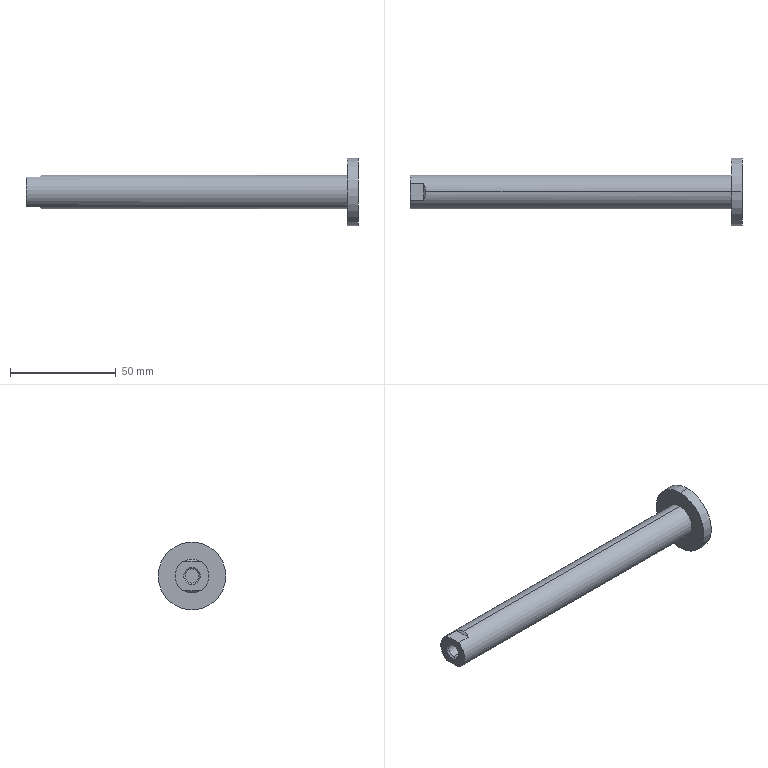Part | STEP file | 2 | 1 solid | 16 faces | box 157 x 32 x 32 mm | volume 34054 mm3 | plane 8 | cylinder 6 | cone 2 | commonest cylinder face diameters 6.647 x2 16 x2 32 x2
STEP:
#1=CARTESIAN_POINT('',(0.,0.,0.));
#2=DIRECTION('',(0.,0.,1.));
#3=DIRECTION('',(1.,0.,0.));
#4=AXIS2_PLACEMENT_3D('',#1,#2,#3);
#5=CARTESIAN_POINT('',(-10.5,3.873,7.));
#6=VERTEX_POINT('',#5);
#7=CARTESIAN_POINT('',(-9.5,0.,8.));
#8=VERTEX_POINT('',#7);
#9=CARTESIAN_POINT('',(-10.5,3.873,7.));
#10=CARTESIAN_POINT('',(-9.841,2.681,7.659));
#11=CARTESIAN_POINT('',(-9.5,1.362,8.));
#12=CARTESIAN_POINT('',(-9.5,0.,8.));
#13=(BOUNDED_CURVE()B_SPLINE_CURVE(3,(#9,#10,#11,#12),.UNSPECIFIED.,.F.,.F.)B_SPLINE_CURVE_WITH_KNOTS((4,4),(5.778,6.283),.PIECEWISE_BEZIER_KNOTS.)CURVE()GEOMETRIC_REPRESENTATION_ITEM()RATIONAL_B_SPLINE_CURVE((1.,0.9788,0.9788,1.))REPRESENTATION_ITEM(''));
#14=CARTESIAN_POINT('',(59.,0.,0.));
#15=DIRECTION('',(1.,0.,0.));
#16=DIRECTION('',(0.,0.,-1.));
#17=AXIS2_PLACEMENT_3D('',#14,#15,#16);
#18=CYLINDRICAL_SURFACE('',#17,8.);
#19=CARTESIAN_POINT('',(2.636,-69.5));
#20=CARTESIAN_POINT('',(2.644,-69.471));
#21=CARTESIAN_POINT('',(2.659,-69.413));
#22=CARTESIAN_POINT('',(2.682,-69.33));
#23=CARTESIAN_POINT('',(2.705,-69.251));
#24=CARTESIAN_POINT('',(2.728,-69.175));
#25=CARTESIAN_POINT('',(2.751,-69.103));
#26=CARTESIAN_POINT('',(2.774,-69.035));
#27=CARTESIAN_POINT('',(2.797,-68.971));
#28=CARTESIAN_POINT('',(2.82,-68.91));
#29=CARTESIAN_POINT('',(2.843,-68.854));
#30=CARTESIAN_POINT('',(2.866,-68.802));
#31=CARTESIAN_POINT('',(2.889,-68.753));
#32=CARTESIAN_POINT('',(2.912,-68.709));
#33=CARTESIAN_POINT('',(2.935,-68.669));
#34=CARTESIAN_POINT('',(2.958,-68.634));
#35=CARTESIAN_POINT('',(2.981,-68.602));
#36=CARTESIAN_POINT('',(3.004,-68.575));
#37=CARTESIAN_POINT('',(3.027,-68.552));
#38=CARTESIAN_POINT('',(3.05,-68.533));
#39=CARTESIAN_POINT('',(3.073,-68.518));
#40=CARTESIAN_POINT('',(3.096,-68.508));
#41=CARTESIAN_POINT('',(3.119,-68.501));
#42=CARTESIAN_POINT('',(3.134,-68.5));
#43=CARTESIAN_POINT('',(3.142,-68.5));
#44=B_SPLINE_CURVE_WITH_KNOTS('',3,(#19,#20,#21,#22,#23,#24,#25,#26,#27,#28,#29,#30,#31,#32,#33,#34,#35,#36,#37,#38,#39,#40,#41,#42,#43),.UNSPECIFIED.,.F.,.F.,(4,1,1,1,1,1,1,1,1,1,1,1,1,1,1,1,1,1,1,1,1,1,4),(5.778,5.801,5.824,5.847,5.87,5.893,5.916,5.939,5.962,5.985,6.008,6.031,6.053,6.076,6.099,6.122,6.145,6.168,6.191,6.214,6.237,6.26,6.283),.QUASI_UNIFORM_KNOTS.);
#45=(GEOMETRIC_REPRESENTATION_CONTEXT(2)PARAMETRIC_REPRESENTATION_CONTEXT()REPRESENTATION_CONTEXT('',''));
#46=DEFINITIONAL_REPRESENTATION('',(#44),#45);
#47=PCURVE('',#18,#46);
#48=CARTESIAN_POINT('',(-5.5,16.,12.));
#49=DIRECTION('',(0.7071,0.,-0.7071));
#50=DIRECTION('',(-0.7071,0.,-0.7071));
#51=AXIS2_PLACEMENT_3D('',#48,#49,#50);
#52=PLANE('',#51);
#53=CARTESIAN_POINT('',(7.071,-12.127));
#54=CARTESIAN_POINT('',(6.138,-13.319));
#55=CARTESIAN_POINT('',(5.657,-14.638));
#56=CARTESIAN_POINT('',(5.657,-16.));
#57=(BOUNDED_CURVE()B_SPLINE_CURVE(3,(#53,#54,#55,#56),.UNSPECIFIED.,.F.,.F.)B_SPLINE_CURVE_WITH_KNOTS((4,4),(5.778,6.283),.PIECEWISE_BEZIER_KNOTS.)CURVE()GEOMETRIC_REPRESENTATION_ITEM()RATIONAL_B_SPLINE_CURVE((1.,0.9788,0.9788,1.))REPRESENTATION_ITEM(''));
#58=(GEOMETRIC_REPRESENTATION_CONTEXT(2)PARAMETRIC_REPRESENTATION_CONTEXT()REPRESENTATION_CONTEXT('',''));
#59=DEFINITIONAL_REPRESENTATION('',(#57),#58);
#60=PCURVE('',#52,#59);
#61=SURFACE_CURVE('',#13,(#47,#60),.PCURVE_S1.);
#62=EDGE_CURVE('',#6,#8,#61,.T.);
#63=ORIENTED_EDGE('',*,*,#62,.T.);
#64=CARTESIAN_POINT('',(135.,0.,8.));
#65=VERTEX_POINT('',#64);
#66=CARTESIAN_POINT('',(59.,0.,8.));
#67=DIRECTION('',(1.,0.,0.));
#68=VECTOR('',#67,1.);
#69=LINE('',#66,#68);
#70=CARTESIAN_POINT('',(3.142,0.));
#71=DIRECTION('',(0.,1.));
#72=VECTOR('',#71,1.);
#73=LINE('',#70,#72);
#74=(GEOMETRIC_REPRESENTATION_CONTEXT(2)PARAMETRIC_REPRESENTATION_CONTEXT()REPRESENTATION_CONTEXT('',''));
#75=DEFINITIONAL_REPRESENTATION('',(#73),#74);
#76=PCURVE('',#18,#75);
#77=CARTESIAN_POINT('',(59.,0.,0.));
#78=DIRECTION('',(1.,0.,0.));
#79=DIRECTION('',(0.,0.,-1.));
#80=AXIS2_PLACEMENT_3D('',#77,#78,#79);
#81=CYLINDRICAL_SURFACE('',#80,8.);
#82=CARTESIAN_POINT('',(3.142,0.));
#83=DIRECTION('',(0.,1.));
#84=VECTOR('',#83,1.);
#85=LINE('',#82,#84);
#86=(GEOMETRIC_REPRESENTATION_CONTEXT(2)PARAMETRIC_REPRESENTATION_CONTEXT()REPRESENTATION_CONTEXT('',''));
#87=DEFINITIONAL_REPRESENTATION('',(#85),#86);
#88=PCURVE('',#81,#87);
#89=SURFACE_CURVE('',#69,(#76,#88),.PCURVE_S1.);
#90=EDGE_CURVE('',#8,#65,#89,.T.);
#91=ORIENTED_EDGE('',*,*,#90,.T.);
#92=CARTESIAN_POINT('',(135.,0.,-8.));
#93=VERTEX_POINT('',#92);
#94=CARTESIAN_POINT('',(135.,0.,0.));
#95=DIRECTION('',(-1.,0.,0.));
#96=DIRECTION('',(0.,0.,-1.));
#97=AXIS2_PLACEMENT_3D('',#94,#95,#96);
#98=CIRCLE('',#97,8.);
#99=CARTESIAN_POINT('',(6.283,76.));
#100=DIRECTION('',(-1.,0.));
#101=VECTOR('',#100,1.);
#102=LINE('',#99,#101);
#103=(GEOMETRIC_REPRESENTATION_CONTEXT(2)PARAMETRIC_REPRESENTATION_CONTEXT()REPRESENTATION_CONTEXT('',''));
#104=DEFINITIONAL_REPRESENTATION('',(#102),#103);
#105=PCURVE('',#18,#104);
#106=CARTESIAN_POINT('',(135.,12.,0.));
#107=DIRECTION('',(-1.,0.,0.));
#108=DIRECTION('',(0.,0.,1.));
#109=AXIS2_PLACEMENT_3D('',#106,#107,#108);
#110=PLANE('',#109);
#111=CARTESIAN_POINT('',(0.,-12.));
#112=DIRECTION('',(-1.,0.));
#113=AXIS2_PLACEMENT_2D('',#111,#112);
#114=CIRCLE('',#113,8.);
#115=(GEOMETRIC_REPRESENTATION_CONTEXT(2)PARAMETRIC_REPRESENTATION_CONTEXT()REPRESENTATION_CONTEXT('',''));
#116=DEFINITIONAL_REPRESENTATION('',(#114),#115);
#117=PCURVE('',#110,#116);
#118=SURFACE_CURVE('',#98,(#105,#117),.PCURVE_S1.);
#119=EDGE_CURVE('',#65,#93,#118,.T.);
#120=ORIENTED_EDGE('',*,*,#119,.T.);
#121=CARTESIAN_POINT('',(-9.5,0.,-8.));
#122=VERTEX_POINT('',#121);
#123=CARTESIAN_POINT('',(59.,0.,-8.));
#124=DIRECTION('',(1.,0.,0.));
#125=VECTOR('',#124,1.);
#126=LINE('',#123,#125);
#127=CARTESIAN_POINT('',(0.,0.));
#128=DIRECTION('',(0.,1.));
#129=VECTOR('',#128,1.);
#130=LINE('',#127,#129);
#131=(GEOMETRIC_REPRESENTATION_CONTEXT(2)PARAMETRIC_REPRESENTATION_CONTEXT()REPRESENTATION_CONTEXT('',''));
#132=DEFINITIONAL_REPRESENTATION('',(#130),#131);
#133=PCURVE('',#18,#132);
#134=CARTESIAN_POINT('',(6.283,0.));
#135=DIRECTION('',(0.,1.));
#136=VECTOR('',#135,1.);
#137=LINE('',#134,#136);
#138=(GEOMETRIC_REPRESENTATION_CONTEXT(2)PARAMETRIC_REPRESENTATION_CONTEXT()REPRESENTATION_CONTEXT('',''));
#139=DEFINITIONAL_REPRESENTATION('',(#137),#138);
#140=PCURVE('',#81,#139);
#141=SURFACE_CURVE('',#126,(#133,#140),.PCURVE_S1.);
#142=EDGE_CURVE('',#122,#93,#141,.T.);
#143=ORIENTED_EDGE('',*,*,#142,.F.);
#144=CARTESIAN_POINT('',(-10.5,3.873,-7.));
#145=VERTEX_POINT('',#144);
#146=CARTESIAN_POINT('',(-9.5,0.,-8.));
#147=CARTESIAN_POINT('',(-9.5,1.362,-8.));
#148=CARTESIAN_POINT('',(-9.841,2.681,-7.659));
#149=CARTESIAN_POINT('',(-10.5,3.873,-7.));
#150=(BOUNDED_CURVE()B_SPLINE_CURVE(3,(#146,#147,#148,#149),.UNSPECIFIED.,.F.,.F.)B_SPLINE_CURVE_WITH_KNOTS((4,4),(0.,0.5054),.PIECEWISE_BEZIER_KNOTS.)CURVE()GEOMETRIC_REPRESENTATION_ITEM()RATIONAL_B_SPLINE_CURVE((1.,0.9788,0.9788,1.))REPRESENTATION_ITEM(''));
#151=CARTESIAN_POINT('',(0.,-68.5));
#152=CARTESIAN_POINT('',(0.007576,-68.5));
#153=CARTESIAN_POINT('',(0.02275,-68.501));
#154=CARTESIAN_POINT('',(0.04557,-68.508));
#155=CARTESIAN_POINT('',(0.06844,-68.518));
#156=CARTESIAN_POINT('',(0.09137,-68.533));
#157=CARTESIAN_POINT('',(0.1143,-68.552));
#158=CARTESIAN_POINT('',(0.1373,-68.575));
#159=CARTESIAN_POINT('',(0.1604,-68.602));
#160=CARTESIAN_POINT('',(0.1834,-68.634));
#161=CARTESIAN_POINT('',(0.2065,-68.669));
#162=CARTESIAN_POINT('',(0.2296,-68.709));
#163=CARTESIAN_POINT('',(0.2527,-68.753));
#164=CARTESIAN_POINT('',(0.2758,-68.802));
#165=CARTESIAN_POINT('',(0.2989,-68.854));
#166=CARTESIAN_POINT('',(0.3219,-68.91));
#167=CARTESIAN_POINT('',(0.345,-68.971));
#168=CARTESIAN_POINT('',(0.368,-69.035));
#169=CARTESIAN_POINT('',(0.391,-69.103));
#170=CARTESIAN_POINT('',(0.414,-69.175));
#171=CARTESIAN_POINT('',(0.4369,-69.251));
#172=CARTESIAN_POINT('',(0.4598,-69.33));
#173=CARTESIAN_POINT('',(0.4826,-69.413));
#174=CARTESIAN_POINT('',(0.4978,-69.471));
#175=CARTESIAN_POINT('',(0.5054,-69.5));
#176=B_SPLINE_CURVE_WITH_KNOTS('',3,(#151,#152,#153,#154,#155,#156,#157,#158,#159,#160,#161,#162,#163,#164,#165,#166,#167,#168,#169,#170,#171,#172,#173,#174,#175),.UNSPECIFIED.,.F.,.F.,(4,1,1,1,1,1,1,1,1,1,1,1,1,1,1,1,1,1,1,1,1,1,4),(0.,0.02297,0.04594,0.06891,0.09188,0.1149,0.1378,0.1608,0.1838,0.2067,0.2297,0.2527,0.2757,0.2986,0.3216,0.3446,0.3675,0.3905,0.4135,0.4364,0.4594,0.4824,0.5054),.QUASI_UNIFORM_KNOTS.);
#177=(GEOMETRIC_REPRESENTATION_CONTEXT(2)PARAMETRIC_REPRESENTATION_CONTEXT()REPRESENTATION_CONTEXT('',''));
#178=DEFINITIONAL_REPRESENTATION('',(#176),#177);
#179=PCURVE('',#18,#178);
#180=CARTESIAN_POINT('',(-10.5,16.,-7.));
#181=DIRECTION('',(0.7071,0.,0.7071));
#182=DIRECTION('',(0.7071,0.,-0.7071));
#183=AXIS2_PLACEMENT_3D('',#180,#181,#182);
#184=PLANE('',#183);
#185=CARTESIAN_POINT('',(1.414,-16.));
#186=CARTESIAN_POINT('',(1.414,-14.638));
#187=CARTESIAN_POINT('',(0.9326,-13.319));
#188=CARTESIAN_POINT('',(0.,-12.127));
#189=(BOUNDED_CURVE()B_SPLINE_CURVE(3,(#185,#186,#187,#188),.UNSPECIFIED.,.F.,.F.)B_SPLINE_CURVE_WITH_KNOTS((4,4),(0.,0.5054),.PIECEWISE_BEZIER_KNOTS.)CURVE()GEOMETRIC_REPRESENTATION_ITEM()RATIONAL_B_SPLINE_CURVE((1.,0.9788,0.9788,1.))REPRESENTATION_ITEM(''));
#190=(GEOMETRIC_REPRESENTATION_CONTEXT(2)PARAMETRIC_REPRESENTATION_CONTEXT()REPRESENTATION_CONTEXT('',''));
#191=DEFINITIONAL_REPRESENTATION('',(#189),#190);
#192=PCURVE('',#184,#191);
#193=SURFACE_CURVE('',#150,(#179,#192),.PCURVE_S1.);
#194=EDGE_CURVE('',#122,#145,#193,.T.);
#195=ORIENTED_EDGE('',*,*,#194,.T.);
#196=CARTESIAN_POINT('',(-17.,3.873,-7.));
#197=VERTEX_POINT('',#196);
#198=CARTESIAN_POINT('',(59.,3.873,-7.));
#199=DIRECTION('',(-1.,0.,0.));
#200=VECTOR('',#199,1.);
#201=LINE('',#198,#200);
#202=CARTESIAN_POINT('',(0.5054,0.));
#203=DIRECTION('',(0.,-1.));
#204=VECTOR('',#203,1.);
#205=LINE('',#202,#204);
#206=(GEOMETRIC_REPRESENTATION_CONTEXT(2)PARAMETRIC_REPRESENTATION_CONTEXT()REPRESENTATION_CONTEXT('',''));
#207=DEFINITIONAL_REPRESENTATION('',(#205),#206);
#208=PCURVE('',#18,#207);
#209=CARTESIAN_POINT('',(-17.,16.,-7.));
#210=DIRECTION('',(0.,0.,1.));
#211=DIRECTION('',(1.,0.,0.));
#212=AXIS2_PLACEMENT_3D('',#209,#210,#211);
#213=PLANE('',#212);
#214=CARTESIAN_POINT('',(76.,-12.127));
#215=DIRECTION('',(-1.,0.));
#216=VECTOR('',#215,1.);
#217=LINE('',#214,#216);
#218=(GEOMETRIC_REPRESENTATION_CONTEXT(2)PARAMETRIC_REPRESENTATION_CONTEXT()REPRESENTATION_CONTEXT('',''));
#219=DEFINITIONAL_REPRESENTATION('',(#217),#218);
#220=PCURVE('',#213,#219);
#221=SURFACE_CURVE('',#201,(#208,#220),.PCURVE_S1.);
#222=EDGE_CURVE('',#145,#197,#221,.T.);
#223=ORIENTED_EDGE('',*,*,#222,.T.);
#224=CARTESIAN_POINT('',(-17.,3.873,7.));
#225=VERTEX_POINT('',#224);
#226=CARTESIAN_POINT('',(-17.,0.,0.));
#227=DIRECTION('',(1.,0.,0.));
#228=DIRECTION('',(0.,0.,-1.));
#229=AXIS2_PLACEMENT_3D('',#226,#227,#228);
#230=CIRCLE('',#229,8.);
#231=CARTESIAN_POINT('',(0.,-76.));
#232=DIRECTION('',(1.,0.));
#233=VECTOR('',#232,1.);
#234=LINE('',#231,#233);
#235=(GEOMETRIC_REPRESENTATION_CONTEXT(2)PARAMETRIC_REPRESENTATION_CONTEXT()REPRESENTATION_CONTEXT('',''));
#236=DEFINITIONAL_REPRESENTATION('',(#234),#235);
#237=PCURVE('',#18,#236);
#238=CARTESIAN_POINT('',(-17.,6.,0.));
#239=DIRECTION('',(-1.,0.,0.));
#240=DIRECTION('',(0.,0.,1.));
#241=AXIS2_PLACEMENT_3D('',#238,#239,#240);
#242=PLANE('',#241);
#243=CARTESIAN_POINT('',(-8.,-6.));
#244=CARTESIAN_POINT('',(-8.,7.856));
#245=CARTESIAN_POINT('',(4.,0.9282));
#246=CARTESIAN_POINT('',(16.,-6.));
#247=CARTESIAN_POINT('',(4.,-12.928));
#248=CARTESIAN_POINT('',(-8.,-19.856));
#249=CARTESIAN_POINT('',(-8.,-6.));
#250=(BOUNDED_CURVE()B_SPLINE_CURVE(2,(#243,#244,#245,#246,#247,#248,#249),.UNSPECIFIED.,.T.,.F.)B_SPLINE_CURVE_WITH_KNOTS((1,2,2,2,2,1),(-2.094,0.,2.094,4.189,6.283,8.378),.UNSPECIFIED.)CURVE()GEOMETRIC_REPRESENTATION_ITEM()RATIONAL_B_SPLINE_CURVE((1.,0.5,1.,0.5,1.,0.5,1.))REPRESENTATION_ITEM(''));
#251=(GEOMETRIC_REPRESENTATION_CONTEXT(2)PARAMETRIC_REPRESENTATION_CONTEXT()REPRESENTATION_CONTEXT('',''));
#252=DEFINITIONAL_REPRESENTATION('',(#250),#251);
#253=PCURVE('',#242,#252);
#254=SURFACE_CURVE('',#230,(#237,#253),.PCURVE_S1.);
#255=EDGE_CURVE('',#197,#225,#254,.T.);
#256=ORIENTED_EDGE('',*,*,#255,.T.);
#257=CARTESIAN_POINT('',(59.,3.873,7.));
#258=DIRECTION('',(1.,0.,0.));
#259=VECTOR('',#258,1.);
#260=LINE('',#257,#259);
#261=CARTESIAN_POINT('',(2.636,0.));
#262=DIRECTION('',(0.,1.));
#263=VECTOR('',#262,1.);
#264=LINE('',#261,#263);
#265=(GEOMETRIC_REPRESENTATION_CONTEXT(2)PARAMETRIC_REPRESENTATION_CONTEXT()REPRESENTATION_CONTEXT('',''));
#266=DEFINITIONAL_REPRESENTATION('',(#264),#265);
#267=PCURVE('',#18,#266);
#268=CARTESIAN_POINT('',(-10.5,16.,7.));
#269=DIRECTION('',(0.,0.,-1.));
#270=DIRECTION('',(-1.,0.,0.));
#271=AXIS2_PLACEMENT_3D('',#268,#269,#270);
#272=PLANE('',#271);
#273=CARTESIAN_POINT('',(-69.5,-12.127));
#274=DIRECTION('',(-1.,0.));
#275=VECTOR('',#274,1.);
#276=LINE('',#273,#275);
#277=(GEOMETRIC_REPRESENTATION_CONTEXT(2)PARAMETRIC_REPRESENTATION_CONTEXT()REPRESENTATION_CONTEXT('',''));
#278=DEFINITIONAL_REPRESENTATION('',(#276),#277);
#279=PCURVE('',#272,#278);
#280=SURFACE_CURVE('',#260,(#267,#279),.PCURVE_S1.);
#281=EDGE_CURVE('',#225,#6,#280,.T.);
#282=ORIENTED_EDGE('',*,*,#281,.T.);
#283=EDGE_LOOP('',(#63,#91,#120,#143,#195,#223,#256,#282));
#284=FACE_BOUND('',#283,.T.);
#285=ADVANCED_FACE('',(#284),#18,.T.);
#286=CARTESIAN_POINT('',(135.,0.,16.));
#287=VERTEX_POINT('',#286);
#288=CARTESIAN_POINT('',(135.,0.,-16.));
#289=VERTEX_POINT('',#288);
#290=CARTESIAN_POINT('',(135.,0.,0.));
#291=DIRECTION('',(-1.,0.,0.));
#292=DIRECTION('',(0.,0.,-1.));
#293=AXIS2_PLACEMENT_3D('',#290,#291,#292);
#294=CIRCLE('',#293,16.);
#295=CARTESIAN_POINT('',(137.5,0.,0.));
#296=DIRECTION('',(1.,0.,0.));
#297=DIRECTION('',(0.,0.,-1.));
#298=AXIS2_PLACEMENT_3D('',#295,#296,#297);
#299=CYLINDRICAL_SURFACE('',#298,16.);
#300=CARTESIAN_POINT('',(6.283,-2.5));
#301=DIRECTION('',(-1.,0.));
#302=VECTOR('',#301,1.);
#303=LINE('',#300,#302);
#304=(GEOMETRIC_REPRESENTATION_CONTEXT(2)PARAMETRIC_REPRESENTATION_CONTEXT()REPRESENTATION_CONTEXT('',''));
#305=DEFINITIONAL_REPRESENTATION('',(#303),#304);
#306=PCURVE('',#299,#305);
#307=CARTESIAN_POINT('',(0.,-12.));
#308=DIRECTION('',(-1.,0.));
#309=AXIS2_PLACEMENT_2D('',#307,#308);
#310=CIRCLE('',#309,16.);
#311=(GEOMETRIC_REPRESENTATION_CONTEXT(2)PARAMETRIC_REPRESENTATION_CONTEXT()REPRESENTATION_CONTEXT('',''));
#312=DEFINITIONAL_REPRESENTATION('',(#310),#311);
#313=PCURVE('',#110,#312);
#314=SURFACE_CURVE('',#294,(#306,#313),.PCURVE_S1.);
#315=EDGE_CURVE('',#287,#289,#314,.T.);
#316=ORIENTED_EDGE('',*,*,#315,.F.);
#317=CARTESIAN_POINT('',(140.,0.,16.));
#318=VERTEX_POINT('',#317);
#319=CARTESIAN_POINT('',(137.5,0.,16.));
#320=DIRECTION('',(1.,0.,0.));
#321=VECTOR('',#320,1.);
#322=LINE('',#319,#321);
#323=CARTESIAN_POINT('',(3.142,0.));
#324=DIRECTION('',(0.,1.));
#325=VECTOR('',#324,1.);
#326=LINE('',#323,#325);
#327=(GEOMETRIC_REPRESENTATION_CONTEXT(2)PARAMETRIC_REPRESENTATION_CONTEXT()REPRESENTATION_CONTEXT('',''));
#328=DEFINITIONAL_REPRESENTATION('',(#326),#327);
#329=PCURVE('',#299,#328);
#330=CARTESIAN_POINT('',(137.5,0.,0.));
#331=DIRECTION('',(1.,0.,0.));
#332=DIRECTION('',(0.,0.,-1.));
#333=AXIS2_PLACEMENT_3D('',#330,#331,#332);
#334=CYLINDRICAL_SURFACE('',#333,16.);
#335=CARTESIAN_POINT('',(3.142,0.));
#336=DIRECTION('',(0.,1.));
#337=VECTOR('',#336,1.);
#338=LINE('',#335,#337);
#339=(GEOMETRIC_REPRESENTATION_CONTEXT(2)PARAMETRIC_REPRESENTATION_CONTEXT()REPRESENTATION_CONTEXT('',''));
#340=DEFINITIONAL_REPRESENTATION('',(#338),#339);
#341=PCURVE('',#334,#340);
#342=SURFACE_CURVE('',#322,(#329,#341),.PCURVE_S1.);
#343=EDGE_CURVE('',#287,#318,#342,.T.);
#344=ORIENTED_EDGE('',*,*,#343,.T.);
#345=CARTESIAN_POINT('',(140.,0.,-16.));
#346=VERTEX_POINT('',#345);
#347=CARTESIAN_POINT('',(140.,0.,0.));
#348=DIRECTION('',(-1.,0.,0.));
#349=DIRECTION('',(0.,0.,-1.));
#350=AXIS2_PLACEMENT_3D('',#347,#348,#349);
#351=CIRCLE('',#350,16.);
#352=CARTESIAN_POINT('',(6.283,2.5));
#353=DIRECTION('',(-1.,0.));
#354=VECTOR('',#353,1.);
#355=LINE('',#352,#354);
#356=(GEOMETRIC_REPRESENTATION_CONTEXT(2)PARAMETRIC_REPRESENTATION_CONTEXT()REPRESENTATION_CONTEXT('',''));
#357=DEFINITIONAL_REPRESENTATION('',(#355),#356);
#358=PCURVE('',#299,#357);
#359=CARTESIAN_POINT('',(140.,8.,0.));
#360=DIRECTION('',(1.,0.,0.));
#361=DIRECTION('',(0.,0.,-1.));
#362=AXIS2_PLACEMENT_3D('',#359,#360,#361);
#363=PLANE('',#362);
#364=CARTESIAN_POINT('',(16.,-8.));
#365=CARTESIAN_POINT('',(16.,-35.713));
#366=CARTESIAN_POINT('',(-8.,-21.856));
#367=CARTESIAN_POINT('',(-32.,-8.));
#368=CARTESIAN_POINT('',(-8.,5.856));
#369=CARTESIAN_POINT('',(16.,19.713));
#370=CARTESIAN_POINT('',(16.,-8.));
#371=(BOUNDED_CURVE()B_SPLINE_CURVE(2,(#364,#365,#366,#367,#368,#369,#370),.UNSPECIFIED.,.T.,.F.)B_SPLINE_CURVE_WITH_KNOTS((1,2,2,2,2,1),(-2.094,0.,2.094,4.189,6.283,8.378),.UNSPECIFIED.)CURVE()GEOMETRIC_REPRESENTATION_ITEM()RATIONAL_B_SPLINE_CURVE((1.,0.5,1.,0.5,1.,0.5,1.))REPRESENTATION_ITEM(''));
#372=(GEOMETRIC_REPRESENTATION_CONTEXT(2)PARAMETRIC_REPRESENTATION_CONTEXT()REPRESENTATION_CONTEXT('',''));
#373=DEFINITIONAL_REPRESENTATION('',(#371),#372);
#374=PCURVE('',#363,#373);
#375=SURFACE_CURVE('',#351,(#358,#374),.PCURVE_S1.);
#376=EDGE_CURVE('',#318,#346,#375,.T.);
#377=ORIENTED_EDGE('',*,*,#376,.T.);
#378=CARTESIAN_POINT('',(137.5,0.,-16.));
#379=DIRECTION('',(1.,0.,0.));
#380=VECTOR('',#379,1.);
#381=LINE('',#378,#380);
#382=CARTESIAN_POINT('',(0.,0.));
#383=DIRECTION('',(0.,1.));
#384=VECTOR('',#383,1.);
#385=LINE('',#382,#384);
#386=(GEOMETRIC_REPRESENTATION_CONTEXT(2)PARAMETRIC_REPRESENTATION_CONTEXT()REPRESENTATION_CONTEXT('',''));
#387=DEFINITIONAL_REPRESENTATION('',(#385),#386);
#388=PCURVE('',#299,#387);
#389=CARTESIAN_POINT('',(6.283,0.));
#390=DIRECTION('',(0.,1.));
#391=VECTOR('',#390,1.);
#392=LINE('',#389,#391);
#393=(GEOMETRIC_REPRESENTATION_CONTEXT(2)PARAMETRIC_REPRESENTATION_CONTEXT()REPRESENTATION_CONTEXT('',''));
#394=DEFINITIONAL_REPRESENTATION('',(#392),#393);
#395=PCURVE('',#334,#394);
#396=SURFACE_CURVE('',#381,(#388,#395),.PCURVE_S1.);
#397=EDGE_CURVE('',#289,#346,#396,.T.);
#398=ORIENTED_EDGE('',*,*,#397,.F.);
#399=EDGE_LOOP('',(#316,#344,#377,#398));
#400=FACE_BOUND('',#399,.T.);
#401=ADVANCED_FACE('',(#400),#299,.T.);
#402=CARTESIAN_POINT('',(-16.323,0.,3.323));
#403=VERTEX_POINT('',#402);
#404=CARTESIAN_POINT('',(-17.,0.,4.));
#405=VERTEX_POINT('',#404);
#406=CARTESIAN_POINT('',(-17.,0.,4.));
#407=DIRECTION('',(-0.7071,0.,0.7071));
#408=VECTOR('',#407,1.);
#409=LINE('',#406,#408);
#410=CARTESIAN_POINT('',(-17.,0.,0.));
#411=DIRECTION('',(-1.,0.,0.));
#412=DIRECTION('',(0.,0.,1.));
#413=AXIS2_PLACEMENT_3D('',#410,#411,#412);
#414=CONICAL_SURFACE('',#413,4.,0.7854);
#415=CARTESIAN_POINT('',(6.283,0.));
#416=DIRECTION('',(0.,1.));
#417=VECTOR('',#416,1.);
#418=LINE('',#415,#417);
#419=(GEOMETRIC_REPRESENTATION_CONTEXT(2)PARAMETRIC_REPRESENTATION_CONTEXT()REPRESENTATION_CONTEXT('',''));
#420=DEFINITIONAL_REPRESENTATION('',(#418),#419);
#421=PCURVE('',#414,#420);
#422=CARTESIAN_POINT('',(-17.,0.,0.));
#423=DIRECTION('',(-1.,0.,0.));
#424=DIRECTION('',(0.,0.,1.));
#425=AXIS2_PLACEMENT_3D('',#422,#423,#424);
#426=CONICAL_SURFACE('',#425,4.,0.7854);
#427=CARTESIAN_POINT('',(0.,0.));
#428=DIRECTION('',(0.,1.));
#429=VECTOR('',#428,1.);
#430=LINE('',#427,#429);
#431=(GEOMETRIC_REPRESENTATION_CONTEXT(2)PARAMETRIC_REPRESENTATION_CONTEXT()REPRESENTATION_CONTEXT('',''));
#432=DEFINITIONAL_REPRESENTATION('',(#430),#431);
#433=PCURVE('',#426,#432);
#434=SURFACE_CURVE('',#409,(#421,#433),.PCURVE_S1.);
#435=EDGE_CURVE('',#403,#405,#434,.T.);
#436=ORIENTED_EDGE('',*,*,#435,.T.);
#437=CARTESIAN_POINT('',(-17.,0.,-4.));
#438=VERTEX_POINT('',#437);
#439=CARTESIAN_POINT('',(-17.,0.,0.));
#440=DIRECTION('',(1.,0.,0.));
#441=DIRECTION('',(0.,0.,1.));
#442=AXIS2_PLACEMENT_3D('',#439,#440,#441);
#443=CIRCLE('',#442,4.);
#444=CARTESIAN_POINT('',(6.283,0.));
#445=DIRECTION('',(-1.,0.));
#446=VECTOR('',#445,1.);
#447=LINE('',#444,#446);
#448=(GEOMETRIC_REPRESENTATION_CONTEXT(2)PARAMETRIC_REPRESENTATION_CONTEXT()REPRESENTATION_CONTEXT('',''));
#449=DEFINITIONAL_REPRESENTATION('',(#447),#448);
#450=PCURVE('',#414,#449);
#451=CARTESIAN_POINT('',(4.,-6.));
#452=CARTESIAN_POINT('',(4.,-12.928));
#453=CARTESIAN_POINT('',(-2.,-9.464));
#454=CARTESIAN_POINT('',(-8.,-6.));
#455=CARTESIAN_POINT('',(-2.,-2.536));
#456=CARTESIAN_POINT('',(4.,0.9282));
#457=CARTESIAN_POINT('',(4.,-6.));
#458=(BOUNDED_CURVE()B_SPLINE_CURVE(2,(#451,#452,#453,#454,#455,#456,#457),.UNSPECIFIED.,.T.,.F.)B_SPLINE_CURVE_WITH_KNOTS((1,2,2,2,2,1),(-2.094,0.,2.094,4.189,6.283,8.378),.UNSPECIFIED.)CURVE()GEOMETRIC_REPRESENTATION_ITEM()RATIONAL_B_SPLINE_CURVE((1.,0.5,1.,0.5,1.,0.5,1.))REPRESENTATION_ITEM(''));
#459=(GEOMETRIC_REPRESENTATION_CONTEXT(2)PARAMETRIC_REPRESENTATION_CONTEXT()REPRESENTATION_CONTEXT('',''));
#460=DEFINITIONAL_REPRESENTATION('',(#458),#459);
#461=PCURVE('',#242,#460);
#462=SURFACE_CURVE('',#443,(#450,#461),.PCURVE_S1.);
#463=EDGE_CURVE('',#405,#438,#462,.T.);
#464=ORIENTED_EDGE('',*,*,#463,.T.);
#465=CARTESIAN_POINT('',(-16.323,0.,-3.323));
#466=VERTEX_POINT('',#465);
#467=CARTESIAN_POINT('',(-17.,0.,-4.));
#468=DIRECTION('',(-0.7071,0.,-0.7071));
#469=VECTOR('',#468,1.);
#470=LINE('',#467,#469);
#471=CARTESIAN_POINT('',(3.142,0.));
#472=DIRECTION('',(0.,1.));
#473=VECTOR('',#472,1.);
#474=LINE('',#471,#473);
#475=(GEOMETRIC_REPRESENTATION_CONTEXT(2)PARAMETRIC_REPRESENTATION_CONTEXT()REPRESENTATION_CONTEXT('',''));
#476=DEFINITIONAL_REPRESENTATION('',(#474),#475);
#477=PCURVE('',#414,#476);
#478=CARTESIAN_POINT('',(3.142,0.));
#479=DIRECTION('',(0.,1.));
#480=VECTOR('',#479,1.);
#481=LINE('',#478,#480);
#482=(GEOMETRIC_REPRESENTATION_CONTEXT(2)PARAMETRIC_REPRESENTATION_CONTEXT()REPRESENTATION_CONTEXT('',''));
#483=DEFINITIONAL_REPRESENTATION('',(#481),#482);
#484=PCURVE('',#426,#483);
#485=SURFACE_CURVE('',#470,(#477,#484),.PCURVE_S1.);
#486=EDGE_CURVE('',#466,#438,#485,.T.);
#487=ORIENTED_EDGE('',*,*,#486,.F.);
#488=CARTESIAN_POINT('',(-16.323,0.,0.));
#489=DIRECTION('',(-1.,0.,0.));
#490=DIRECTION('',(0.,1.,0.));
#491=AXIS2_PLACEMENT_3D('',#488,#489,#490);
#492=CIRCLE('',#491,3.323);
#493=CARTESIAN_POINT('',(1.571,-0.6765));
#494=DIRECTION('',(1.,0.));
#495=VECTOR('',#494,1.);
#496=LINE('',#493,#495);
#497=(GEOMETRIC_REPRESENTATION_CONTEXT(2)PARAMETRIC_REPRESENTATION_CONTEXT()REPRESENTATION_CONTEXT('',''));
#498=DEFINITIONAL_REPRESENTATION('',(#496),#497);
#499=PCURVE('',#414,#498);
#500=CARTESIAN_POINT('',(-10.162,0.,0.));
#501=DIRECTION('',(1.,0.,0.));
#502=DIRECTION('',(0.,0.,-1.));
#503=AXIS2_PLACEMENT_3D('',#500,#501,#502);
#504=CYLINDRICAL_SURFACE('',#503,3.324);
#505=CARTESIAN_POINT('',(7.854,-6.162));
#506=DIRECTION('',(-1.,0.));
#507=VECTOR('',#506,1.);
#508=LINE('',#505,#507);
#509=(GEOMETRIC_REPRESENTATION_CONTEXT(2)PARAMETRIC_REPRESENTATION_CONTEXT()REPRESENTATION_CONTEXT('',''));
#510=DEFINITIONAL_REPRESENTATION('',(#508),#509);
#511=PCURVE('',#504,#510);
#512=SURFACE_CURVE('',#492,(#499,#511),.PCURVE_S1.);
#513=EDGE_CURVE('',#466,#403,#512,.T.);
#514=ORIENTED_EDGE('',*,*,#513,.T.);
#515=EDGE_LOOP('',(#436,#464,#487,#514));
#516=FACE_BOUND('',#515,.F.);
#517=ADVANCED_FACE('',(#516),#414,.F.);
#518=CARTESIAN_POINT('',(-4.,0.,-3.324));
#519=VERTEX_POINT('',#518);
#520=CARTESIAN_POINT('',(-10.162,0.,-3.324));
#521=DIRECTION('',(1.,0.,0.));
#522=VECTOR('',#521,1.);
#523=LINE('',#520,#522);
#524=CARTESIAN_POINT('',(6.283,0.));
#525=DIRECTION('',(0.,1.));
#526=VECTOR('',#525,1.);
#527=LINE('',#524,#526);
#528=(GEOMETRIC_REPRESENTATION_CONTEXT(2)PARAMETRIC_REPRESENTATION_CONTEXT()REPRESENTATION_CONTEXT('',''));
#529=DEFINITIONAL_REPRESENTATION('',(#527),#528);
#530=PCURVE('',#504,#529);
#531=CARTESIAN_POINT('',(-10.162,0.,0.));
#532=DIRECTION('',(1.,0.,0.));
#533=DIRECTION('',(0.,0.,-1.));
#534=AXIS2_PLACEMENT_3D('',#531,#532,#533);
#535=CYLINDRICAL_SURFACE('',#534,3.324);
#536=CARTESIAN_POINT('',(0.,0.));
#537=DIRECTION('',(0.,1.));
#538=VECTOR('',#537,1.);
#539=LINE('',#536,#538);
#540=(GEOMETRIC_REPRESENTATION_CONTEXT(2)PARAMETRIC_REPRESENTATION_CONTEXT()REPRESENTATION_CONTEXT('',''));
#541=DEFINITIONAL_REPRESENTATION('',(#539),#540);
#542=PCURVE('',#535,#541);
#543=SURFACE_CURVE('',#523,(#530,#542),.PCURVE_S1.);
#544=EDGE_CURVE('',#466,#519,#543,.T.);
#545=ORIENTED_EDGE('',*,*,#544,.T.);
#546=CARTESIAN_POINT('',(-4.,0.,3.324));
#547=VERTEX_POINT('',#546);
#548=CARTESIAN_POINT('',(-4.,0.,0.));
#549=DIRECTION('',(-1.,0.,0.));
#550=DIRECTION('',(0.,0.,-1.));
#551=AXIS2_PLACEMENT_3D('',#548,#549,#550);
#552=CIRCLE('',#551,3.324);
#553=CARTESIAN_POINT('',(6.283,6.162));
#554=DIRECTION('',(-1.,0.));
#555=VECTOR('',#554,1.);
#556=LINE('',#553,#555);
#557=(GEOMETRIC_REPRESENTATION_CONTEXT(2)PARAMETRIC_REPRESENTATION_CONTEXT()REPRESENTATION_CONTEXT('',''));
#558=DEFINITIONAL_REPRESENTATION('',(#556),#557);
#559=PCURVE('',#504,#558);
#560=CARTESIAN_POINT('',(-4.,1.662,0.));
#561=DIRECTION('',(-1.,0.,0.));
#562=DIRECTION('',(0.,0.,1.));
#563=AXIS2_PLACEMENT_3D('',#560,#561,#562);
#564=PLANE('',#563);
#565=CARTESIAN_POINT('',(0.,-1.662));
#566=DIRECTION('',(-1.,0.));
#567=AXIS2_PLACEMENT_2D('',#565,#566);
#568=CIRCLE('',#567,3.324);
#569=(GEOMETRIC_REPRESENTATION_CONTEXT(2)PARAMETRIC_REPRESENTATION_CONTEXT()REPRESENTATION_CONTEXT('',''));
#570=DEFINITIONAL_REPRESENTATION('',(#568),#569);
#571=PCURVE('',#564,#570);
#572=SURFACE_CURVE('',#552,(#559,#571),.PCURVE_S1.);
#573=EDGE_CURVE('',#519,#547,#572,.T.);
#574=ORIENTED_EDGE('',*,*,#573,.T.);
#575=CARTESIAN_POINT('',(-10.162,0.,3.324));
#576=DIRECTION('',(1.,0.,0.));
#577=VECTOR('',#576,1.);
#578=LINE('',#575,#577);
#579=CARTESIAN_POINT('',(3.142,0.));
#580=DIRECTION('',(0.,1.));
#581=VECTOR('',#580,1.);
#582=LINE('',#579,#581);
#583=(GEOMETRIC_REPRESENTATION_CONTEXT(2)PARAMETRIC_REPRESENTATION_CONTEXT()REPRESENTATION_CONTEXT('',''));
#584=DEFINITIONAL_REPRESENTATION('',(#582),#583);
#585=PCURVE('',#504,#584);
#586=CARTESIAN_POINT('',(3.142,0.));
#587=DIRECTION('',(0.,1.));
#588=VECTOR('',#587,1.);
#589=LINE('',#586,#588);
#590=(GEOMETRIC_REPRESENTATION_CONTEXT(2)PARAMETRIC_REPRESENTATION_CONTEXT()REPRESENTATION_CONTEXT('',''));
#591=DEFINITIONAL_REPRESENTATION('',(#589),#590);
#592=PCURVE('',#535,#591);
#593=SURFACE_CURVE('',#578,(#585,#592),.PCURVE_S1.);
#594=EDGE_CURVE('',#403,#547,#593,.T.);
#595=ORIENTED_EDGE('',*,*,#594,.F.);
#596=ORIENTED_EDGE('',*,*,#513,.F.);
#597=EDGE_LOOP('',(#545,#574,#595,#596));
#598=FACE_BOUND('',#597,.F.);
#599=ADVANCED_FACE('',(#598),#504,.F.);
#600=ORIENTED_EDGE('',*,*,#90,.F.);
#601=CARTESIAN_POINT('',(-10.5,-3.873,7.));
#602=VERTEX_POINT('',#601);
#603=CARTESIAN_POINT('',(-9.5,0.,8.));
#604=CARTESIAN_POINT('',(-9.5,-1.362,8.));
#605=CARTESIAN_POINT('',(-9.841,-2.681,7.659));
#606=CARTESIAN_POINT('',(-10.5,-3.873,7.));
#607=(BOUNDED_CURVE()B_SPLINE_CURVE(3,(#603,#604,#605,#606),.UNSPECIFIED.,.F.,.F.)B_SPLINE_CURVE_WITH_KNOTS((4,4),(0.,0.5054),.PIECEWISE_BEZIER_KNOTS.)CURVE()GEOMETRIC_REPRESENTATION_ITEM()RATIONAL_B_SPLINE_CURVE((1.,0.9788,0.9788,1.))REPRESENTATION_ITEM(''));
#608=CARTESIAN_POINT('',(3.142,-68.5));
#609=CARTESIAN_POINT('',(3.149,-68.5));
#610=CARTESIAN_POINT('',(3.164,-68.501));
#611=CARTESIAN_POINT('',(3.187,-68.508));
#612=CARTESIAN_POINT('',(3.21,-68.518));
#613=CARTESIAN_POINT('',(3.233,-68.533));
#614=CARTESIAN_POINT('',(3.256,-68.552));
#615=CARTESIAN_POINT('',(3.279,-68.575));
#616=CARTESIAN_POINT('',(3.302,-68.602));
#617=CARTESIAN_POINT('',(3.325,-68.634));
#618=CARTESIAN_POINT('',(3.348,-68.669));
#619=CARTESIAN_POINT('',(3.371,-68.709));
#620=CARTESIAN_POINT('',(3.394,-68.753));
#621=CARTESIAN_POINT('',(3.417,-68.802));
#622=CARTESIAN_POINT('',(3.44,-68.854));
#623=CARTESIAN_POINT('',(3.464,-68.91));
#624=CARTESIAN_POINT('',(3.487,-68.971));
#625=CARTESIAN_POINT('',(3.51,-69.035));
#626=CARTESIAN_POINT('',(3.533,-69.103));
#627=CARTESIAN_POINT('',(3.556,-69.175));
#628=CARTESIAN_POINT('',(3.579,-69.251));
#629=CARTESIAN_POINT('',(3.601,-69.33));
#630=CARTESIAN_POINT('',(3.624,-69.413));
#631=CARTESIAN_POINT('',(3.639,-69.471));
#632=CARTESIAN_POINT('',(3.647,-69.5));
#633=B_SPLINE_CURVE_WITH_KNOTS('',3,(#608,#609,#610,#611,#612,#613,#614,#615,#616,#617,#618,#619,#620,#621,#622,#623,#624,#625,#626,#627,#628,#629,#630,#631,#632),.UNSPECIFIED.,.F.,.F.,(4,1,1,1,1,1,1,1,1,1,1,1,1,1,1,1,1,1,1,1,1,1,4),(0.,0.02297,0.04594,0.06891,0.09188,0.1149,0.1378,0.1608,0.1838,0.2067,0.2297,0.2527,0.2757,0.2986,0.3216,0.3446,0.3675,0.3905,0.4135,0.4364,0.4594,0.4824,0.5054),.QUASI_UNIFORM_KNOTS.);
#634=(GEOMETRIC_REPRESENTATION_CONTEXT(2)PARAMETRIC_REPRESENTATION_CONTEXT()REPRESENTATION_CONTEXT('',''));
#635=DEFINITIONAL_REPRESENTATION('',(#633),#634);
#636=PCURVE('',#81,#635);
#637=CARTESIAN_POINT('',(5.657,-16.));
#638=CARTESIAN_POINT('',(5.657,-17.362));
#639=CARTESIAN_POINT('',(6.138,-18.681));
#640=CARTESIAN_POINT('',(7.071,-19.873));
#641=(BOUNDED_CURVE()B_SPLINE_CURVE(3,(#637,#638,#639,#640),.UNSPECIFIED.,.F.,.F.)B_SPLINE_CURVE_WITH_KNOTS((4,4),(0.,0.5054),.PIECEWISE_BEZIER_KNOTS.)CURVE()GEOMETRIC_REPRESENTATION_ITEM()RATIONAL_B_SPLINE_CURVE((1.,0.9788,0.9788,1.))REPRESENTATION_ITEM(''));
#642=(GEOMETRIC_REPRESENTATION_CONTEXT(2)PARAMETRIC_REPRESENTATION_CONTEXT()REPRESENTATION_CONTEXT('',''));
#643=DEFINITIONAL_REPRESENTATION('',(#641),#642);
#644=PCURVE('',#52,#643);
#645=SURFACE_CURVE('',#607,(#636,#644),.PCURVE_S1.);
#646=EDGE_CURVE('',#8,#602,#645,.T.);
#647=ORIENTED_EDGE('',*,*,#646,.T.);
#648=CARTESIAN_POINT('',(-17.,-3.873,7.));
#649=VERTEX_POINT('',#648);
#650=CARTESIAN_POINT('',(59.,-3.873,7.));
#651=DIRECTION('',(-1.,0.,0.));
#652=VECTOR('',#651,1.);
#653=LINE('',#650,#652);
#654=CARTESIAN_POINT('',(3.647,0.));
#655=DIRECTION('',(0.,-1.));
#656=VECTOR('',#655,1.);
#657=LINE('',#654,#656);
#658=(GEOMETRIC_REPRESENTATION_CONTEXT(2)PARAMETRIC_REPRESENTATION_CONTEXT()REPRESENTATION_CONTEXT('',''));
#659=DEFINITIONAL_REPRESENTATION('',(#657),#658);
#660=PCURVE('',#81,#659);
#661=CARTESIAN_POINT('',(-69.5,-19.873));
#662=DIRECTION('',(1.,0.));
#663=VECTOR('',#662,1.);
#664=LINE('',#661,#663);
#665=(GEOMETRIC_REPRESENTATION_CONTEXT(2)PARAMETRIC_REPRESENTATION_CONTEXT()REPRESENTATION_CONTEXT('',''));
#666=DEFINITIONAL_REPRESENTATION('',(#664),#665);
#667=PCURVE('',#272,#666);
#668=SURFACE_CURVE('',#653,(#660,#667),.PCURVE_S1.);
#669=EDGE_CURVE('',#602,#649,#668,.T.);
#670=ORIENTED_EDGE('',*,*,#669,.T.);
#671=CARTESIAN_POINT('',(-17.,-3.873,-7.));
#672=VERTEX_POINT('',#671);
#673=CARTESIAN_POINT('',(-17.,0.,0.));
#674=DIRECTION('',(1.,0.,0.));
#675=DIRECTION('',(0.,0.,-1.));
#676=AXIS2_PLACEMENT_3D('',#673,#674,#675);
#677=CIRCLE('',#676,8.);
#678=CARTESIAN_POINT('',(0.,-76.));
#679=DIRECTION('',(1.,0.));
#680=VECTOR('',#679,1.);
#681=LINE('',#678,#680);
#682=(GEOMETRIC_REPRESENTATION_CONTEXT(2)PARAMETRIC_REPRESENTATION_CONTEXT()REPRESENTATION_CONTEXT('',''));
#683=DEFINITIONAL_REPRESENTATION('',(#681),#682);
#684=PCURVE('',#81,#683);
#685=CARTESIAN_POINT('',(-8.,-6.));
#686=CARTESIAN_POINT('',(-8.,7.856));
#687=CARTESIAN_POINT('',(4.,0.9282));
#688=CARTESIAN_POINT('',(16.,-6.));
#689=CARTESIAN_POINT('',(4.,-12.928));
#690=CARTESIAN_POINT('',(-8.,-19.856));
#691=CARTESIAN_POINT('',(-8.,-6.));
#692=(BOUNDED_CURVE()B_SPLINE_CURVE(2,(#685,#686,#687,#688,#689,#690,#691),.UNSPECIFIED.,.T.,.F.)B_SPLINE_CURVE_WITH_KNOTS((1,2,2,2,2,1),(-2.094,0.,2.094,4.189,6.283,8.378),.UNSPECIFIED.)CURVE()GEOMETRIC_REPRESENTATION_ITEM()RATIONAL_B_SPLINE_CURVE((1.,0.5,1.,0.5,1.,0.5,1.))REPRESENTATION_ITEM(''));
#693=(GEOMETRIC_REPRESENTATION_CONTEXT(2)PARAMETRIC_REPRESENTATION_CONTEXT()REPRESENTATION_CONTEXT('',''));
#694=DEFINITIONAL_REPRESENTATION('',(#692),#693);
#695=PCURVE('',#242,#694);
#696=SURFACE_CURVE('',#677,(#684,#695),.PCURVE_S1.);
#697=EDGE_CURVE('',#649,#672,#696,.T.);
#698=ORIENTED_EDGE('',*,*,#697,.T.);
#699=CARTESIAN_POINT('',(-10.5,-3.873,-7.));
#700=VERTEX_POINT('',#699);
#701=CARTESIAN_POINT('',(59.,-3.873,-7.));
#702=DIRECTION('',(1.,0.,0.));
#703=VECTOR('',#702,1.);
#704=LINE('',#701,#703);
#705=CARTESIAN_POINT('',(5.778,0.));
#706=DIRECTION('',(0.,1.));
#707=VECTOR('',#706,1.);
#708=LINE('',#705,#707);
#709=(GEOMETRIC_REPRESENTATION_CONTEXT(2)PARAMETRIC_REPRESENTATION_CONTEXT()REPRESENTATION_CONTEXT('',''));
#710=DEFINITIONAL_REPRESENTATION('',(#708),#709);
#711=PCURVE('',#81,#710);
#712=CARTESIAN_POINT('',(76.,-19.873));
#713=DIRECTION('',(1.,0.));
#714=VECTOR('',#713,1.);
#715=LINE('',#712,#714);
#716=(GEOMETRIC_REPRESENTATION_CONTEXT(2)PARAMETRIC_REPRESENTATION_CONTEXT()REPRESENTATION_CONTEXT('',''));
#717=DEFINITIONAL_REPRESENTATION('',(#715),#716);
#718=PCURVE('',#213,#717);
#719=SURFACE_CURVE('',#704,(#711,#718),.PCURVE_S1.);
#720=EDGE_CURVE('',#672,#700,#719,.T.);
#721=ORIENTED_EDGE('',*,*,#720,.T.);
#722=CARTESIAN_POINT('',(-10.5,-3.873,-7.));
#723=CARTESIAN_POINT('',(-9.841,-2.681,-7.659));
#724=CARTESIAN_POINT('',(-9.5,-1.362,-8.));
#725=CARTESIAN_POINT('',(-9.5,0.,-8.));
#726=(BOUNDED_CURVE()B_SPLINE_CURVE(3,(#722,#723,#724,#725),.UNSPECIFIED.,.F.,.F.)B_SPLINE_CURVE_WITH_KNOTS((4,4),(5.778,6.283),.PIECEWISE_BEZIER_KNOTS.)CURVE()GEOMETRIC_REPRESENTATION_ITEM()RATIONAL_B_SPLINE_CURVE((1.,0.9788,0.9788,1.))REPRESENTATION_ITEM(''));
#727=CARTESIAN_POINT('',(5.778,-69.5));
#728=CARTESIAN_POINT('',(5.785,-69.471));
#729=CARTESIAN_POINT('',(5.801,-69.413));
#730=CARTESIAN_POINT('',(5.823,-69.33));
#731=CARTESIAN_POINT('',(5.846,-69.251));
#732=CARTESIAN_POINT('',(5.869,-69.175));
#733=CARTESIAN_POINT('',(5.892,-69.103));
#734=CARTESIAN_POINT('',(5.915,-69.035));
#735=CARTESIAN_POINT('',(5.938,-68.971));
#736=CARTESIAN_POINT('',(5.961,-68.91));
#737=CARTESIAN_POINT('',(5.984,-68.854));
#738=CARTESIAN_POINT('',(6.007,-68.802));
#739=CARTESIAN_POINT('',(6.031,-68.753));
#740=CARTESIAN_POINT('',(6.054,-68.709));
#741=CARTESIAN_POINT('',(6.077,-68.669));
#742=CARTESIAN_POINT('',(6.1,-68.634));
#743=CARTESIAN_POINT('',(6.123,-68.602));
#744=CARTESIAN_POINT('',(6.146,-68.575));
#745=CARTESIAN_POINT('',(6.169,-68.552));
#746=CARTESIAN_POINT('',(6.192,-68.533));
#747=CARTESIAN_POINT('',(6.215,-68.518));
#748=CARTESIAN_POINT('',(6.238,-68.508));
#749=CARTESIAN_POINT('',(6.26,-68.501));
#750=CARTESIAN_POINT('',(6.276,-68.5));
#751=CARTESIAN_POINT('',(6.283,-68.5));
#752=B_SPLINE_CURVE_WITH_KNOTS('',3,(#727,#728,#729,#730,#731,#732,#733,#734,#735,#736,#737,#738,#739,#740,#741,#742,#743,#744,#745,#746,#747,#748,#749,#750,#751),.UNSPECIFIED.,.F.,.F.,(4,1,1,1,1,1,1,1,1,1,1,1,1,1,1,1,1,1,1,1,1,1,4),(5.778,5.801,5.824,5.847,5.87,5.893,5.916,5.939,5.962,5.985,6.008,6.031,6.053,6.076,6.099,6.122,6.145,6.168,6.191,6.214,6.237,6.26,6.283),.QUASI_UNIFORM_KNOTS.);
#753=(GEOMETRIC_REPRESENTATION_CONTEXT(2)PARAMETRIC_REPRESENTATION_CONTEXT()REPRESENTATION_CONTEXT('',''));
#754=DEFINITIONAL_REPRESENTATION('',(#752),#753);
#755=PCURVE('',#81,#754);
#756=CARTESIAN_POINT('',(0.,-19.873));
#757=CARTESIAN_POINT('',(0.9326,-18.681));
#758=CARTESIAN_POINT('',(1.414,-17.362));
#759=CARTESIAN_POINT('',(1.414,-16.));
#760=(BOUNDED_CURVE()B_SPLINE_CURVE(3,(#756,#757,#758,#759),.UNSPECIFIED.,.F.,.F.)B_SPLINE_CURVE_WITH_KNOTS((4,4),(5.778,6.283),.PIECEWISE_BEZIER_KNOTS.)CURVE()GEOMETRIC_REPRESENTATION_ITEM()RATIONAL_B_SPLINE_CURVE((1.,0.9788,0.9788,1.))REPRESENTATION_ITEM(''));
#761=(GEOMETRIC_REPRESENTATION_CONTEXT(2)PARAMETRIC_REPRESENTATION_CONTEXT()REPRESENTATION_CONTEXT('',''));
#762=DEFINITIONAL_REPRESENTATION('',(#760),#761);
#763=PCURVE('',#184,#762);
#764=SURFACE_CURVE('',#726,(#755,#763),.PCURVE_S1.);
#765=EDGE_CURVE('',#700,#122,#764,.T.);
#766=ORIENTED_EDGE('',*,*,#765,.T.);
#767=ORIENTED_EDGE('',*,*,#142,.T.);
#768=CARTESIAN_POINT('',(135.,0.,0.));
#769=DIRECTION('',(-1.,0.,0.));
#770=DIRECTION('',(0.,0.,-1.));
#771=AXIS2_PLACEMENT_3D('',#768,#769,#770);
#772=CIRCLE('',#771,8.);
#773=CARTESIAN_POINT('',(6.283,76.));
#774=DIRECTION('',(-1.,0.));
#775=VECTOR('',#774,1.);
#776=LINE('',#773,#775);
#777=(GEOMETRIC_REPRESENTATION_CONTEXT(2)PARAMETRIC_REPRESENTATION_CONTEXT()REPRESENTATION_CONTEXT('',''));
#778=DEFINITIONAL_REPRESENTATION('',(#776),#777);
#779=PCURVE('',#81,#778);
#780=CARTESIAN_POINT('',(0.,-12.));
#781=DIRECTION('',(-1.,0.));
#782=AXIS2_PLACEMENT_2D('',#780,#781);
#783=CIRCLE('',#782,8.);
#784=(GEOMETRIC_REPRESENTATION_CONTEXT(2)PARAMETRIC_REPRESENTATION_CONTEXT()REPRESENTATION_CONTEXT('',''));
#785=DEFINITIONAL_REPRESENTATION('',(#783),#784);
#786=PCURVE('',#110,#785);
#787=SURFACE_CURVE('',#772,(#779,#786),.PCURVE_S1.);
#788=EDGE_CURVE('',#93,#65,#787,.T.);
#789=ORIENTED_EDGE('',*,*,#788,.T.);
#790=EDGE_LOOP('',(#600,#647,#670,#698,#721,#766,#767,#789));
#791=FACE_BOUND('',#790,.T.);
#792=ADVANCED_FACE('',(#791),#81,.T.);
#793=CARTESIAN_POINT('',(135.,0.,0.));
#794=DIRECTION('',(-1.,0.,0.));
#795=DIRECTION('',(0.,0.,-1.));
#796=AXIS2_PLACEMENT_3D('',#793,#794,#795);
#797=CIRCLE('',#796,16.);
#798=CARTESIAN_POINT('',(0.,-12.));
#799=DIRECTION('',(-1.,0.));
#800=AXIS2_PLACEMENT_2D('',#798,#799);
#801=CIRCLE('',#800,16.);
#802=(GEOMETRIC_REPRESENTATION_CONTEXT(2)PARAMETRIC_REPRESENTATION_CONTEXT()REPRESENTATION_CONTEXT('',''));
#803=DEFINITIONAL_REPRESENTATION('',(#801),#802);
#804=PCURVE('',#110,#803);
#805=CARTESIAN_POINT('',(6.283,-2.5));
#806=DIRECTION('',(-1.,0.));
#807=VECTOR('',#806,1.);
#808=LINE('',#805,#807);
#809=(GEOMETRIC_REPRESENTATION_CONTEXT(2)PARAMETRIC_REPRESENTATION_CONTEXT()REPRESENTATION_CONTEXT('',''));
#810=DEFINITIONAL_REPRESENTATION('',(#808),#809);
#811=PCURVE('',#334,#810);
#812=SURFACE_CURVE('',#797,(#804,#811),.PCURVE_S1.);
#813=EDGE_CURVE('',#289,#287,#812,.T.);
#814=ORIENTED_EDGE('',*,*,#813,.T.);
#815=ORIENTED_EDGE('',*,*,#315,.T.);
#816=EDGE_LOOP('',(#814,#815));
#817=FACE_BOUND('',#816,.T.);
#818=ORIENTED_EDGE('',*,*,#788,.F.);
#819=ORIENTED_EDGE('',*,*,#119,.F.);
#820=EDGE_LOOP('',(#818,#819));
#821=FACE_BOUND('',#820,.T.);
#822=ADVANCED_FACE('',(#817,#821),#110,.T.);
#823=CARTESIAN_POINT('',(-17.,6.,-7.));
#824=DIRECTION('',(0.,-1.,0.));
#825=VECTOR('',#824,1.);
#826=LINE('',#823,#825);
#827=CARTESIAN_POINT('',(-7.,0.));
#828=DIRECTION('',(0.,-1.));
#829=VECTOR('',#828,1.);
#830=LINE('',#827,#829);
#831=(GEOMETRIC_REPRESENTATION_CONTEXT(2)PARAMETRIC_REPRESENTATION_CONTEXT()REPRESENTATION_CONTEXT('',''));
#832=DEFINITIONAL_REPRESENTATION('',(#830),#831);
#833=PCURVE('',#242,#832);
#834=CARTESIAN_POINT('',(0.,-10.));
#835=DIRECTION('',(0.,-1.));
#836=VECTOR('',#835,1.);
#837=LINE('',#834,#836);
#838=(GEOMETRIC_REPRESENTATION_CONTEXT(2)PARAMETRIC_REPRESENTATION_CONTEXT()REPRESENTATION_CONTEXT('',''));
#839=DEFINITIONAL_REPRESENTATION('',(#837),#838);
#840=PCURVE('',#213,#839);
#841=SURFACE_CURVE('',#826,(#833,#840),.PCURVE_S1.);
#842=EDGE_CURVE('',#197,#672,#841,.T.);
#843=ORIENTED_EDGE('',*,*,#842,.T.);
#844=ORIENTED_EDGE('',*,*,#697,.F.);
#845=CARTESIAN_POINT('',(-17.,6.,7.));
#846=DIRECTION('',(0.,1.,0.));
#847=VECTOR('',#846,1.);
#848=LINE('',#845,#847);
#849=CARTESIAN_POINT('',(7.,0.));
#850=DIRECTION('',(0.,1.));
#851=VECTOR('',#850,1.);
#852=LINE('',#849,#851);
#853=(GEOMETRIC_REPRESENTATION_CONTEXT(2)PARAMETRIC_REPRESENTATION_CONTEXT()REPRESENTATION_CONTEXT('',''));
#854=DEFINITIONAL_REPRESENTATION('',(#852),#853);
#855=PCURVE('',#242,#854);
#856=CARTESIAN_POINT('',(6.5,-10.));
#857=DIRECTION('',(0.,1.));
#858=VECTOR('',#857,1.);
#859=LINE('',#856,#858);
#860=(GEOMETRIC_REPRESENTATION_CONTEXT(2)PARAMETRIC_REPRESENTATION_CONTEXT()REPRESENTATION_CONTEXT('',''));
#861=DEFINITIONAL_REPRESENTATION('',(#859),#860);
#862=PCURVE('',#272,#861);
#863=SURFACE_CURVE('',#848,(#855,#862),.PCURVE_S1.);
#864=EDGE_CURVE('',#649,#225,#863,.T.);
#865=ORIENTED_EDGE('',*,*,#864,.T.);
#866=ORIENTED_EDGE('',*,*,#255,.F.);
#867=EDGE_LOOP('',(#843,#844,#865,#866));
#868=FACE_BOUND('',#867,.T.);
#869=ORIENTED_EDGE('',*,*,#463,.T.);
#870=CARTESIAN_POINT('',(-17.,0.,0.));
#871=DIRECTION('',(1.,0.,0.));
#872=DIRECTION('',(0.,0.,1.));
#873=AXIS2_PLACEMENT_3D('',#870,#871,#872);
#874=CIRCLE('',#873,4.);
#875=CARTESIAN_POINT('',(4.,-6.));
#876=CARTESIAN_POINT('',(4.,-12.928));
#877=CARTESIAN_POINT('',(-2.,-9.464));
#878=CARTESIAN_POINT('',(-8.,-6.));
#879=CARTESIAN_POINT('',(-2.,-2.536));
#880=CARTESIAN_POINT('',(4.,0.9282));
#881=CARTESIAN_POINT('',(4.,-6.));
#882=(BOUNDED_CURVE()B_SPLINE_CURVE(2,(#875,#876,#877,#878,#879,#880,#881),.UNSPECIFIED.,.T.,.F.)B_SPLINE_CURVE_WITH_KNOTS((1,2,2,2,2,1),(-2.094,0.,2.094,4.189,6.283,8.378),.UNSPECIFIED.)CURVE()GEOMETRIC_REPRESENTATION_ITEM()RATIONAL_B_SPLINE_CURVE((1.,0.5,1.,0.5,1.,0.5,1.))REPRESENTATION_ITEM(''));
#883=(GEOMETRIC_REPRESENTATION_CONTEXT(2)PARAMETRIC_REPRESENTATION_CONTEXT()REPRESENTATION_CONTEXT('',''));
#884=DEFINITIONAL_REPRESENTATION('',(#882),#883);
#885=PCURVE('',#242,#884);
#886=CARTESIAN_POINT('',(6.283,0.));
#887=DIRECTION('',(-1.,0.));
#888=VECTOR('',#887,1.);
#889=LINE('',#886,#888);
#890=(GEOMETRIC_REPRESENTATION_CONTEXT(2)PARAMETRIC_REPRESENTATION_CONTEXT()REPRESENTATION_CONTEXT('',''));
#891=DEFINITIONAL_REPRESENTATION('',(#889),#890);
#892=PCURVE('',#426,#891);
#893=SURFACE_CURVE('',#874,(#885,#892),.PCURVE_S1.);
#894=EDGE_CURVE('',#438,#405,#893,.T.);
#895=ORIENTED_EDGE('',*,*,#894,.T.);
#896=EDGE_LOOP('',(#869,#895));
#897=FACE_BOUND('',#896,.T.);
#898=ADVANCED_FACE('',(#868,#897),#242,.T.);
#899=CARTESIAN_POINT('',(-10.5,16.,7.));
#900=DIRECTION('',(0.,-1.,0.));
#901=VECTOR('',#900,1.);
#902=LINE('',#899,#901);
#903=CARTESIAN_POINT('',(0.,0.));
#904=DIRECTION('',(0.,-1.));
#905=VECTOR('',#904,1.);
#906=LINE('',#903,#905);
#907=(GEOMETRIC_REPRESENTATION_CONTEXT(2)PARAMETRIC_REPRESENTATION_CONTEXT()REPRESENTATION_CONTEXT('',''));
#908=DEFINITIONAL_REPRESENTATION('',(#906),#907);
#909=PCURVE('',#272,#908);
#910=CARTESIAN_POINT('',(7.071,0.));
#911=DIRECTION('',(0.,-1.));
#912=VECTOR('',#911,1.);
#913=LINE('',#910,#912);
#914=(GEOMETRIC_REPRESENTATION_CONTEXT(2)PARAMETRIC_REPRESENTATION_CONTEXT()REPRESENTATION_CONTEXT('',''));
#915=DEFINITIONAL_REPRESENTATION('',(#913),#914);
#916=PCURVE('',#52,#915);
#917=SURFACE_CURVE('',#902,(#909,#916),.PCURVE_S1.);
#918=EDGE_CURVE('',#6,#602,#917,.T.);
#919=ORIENTED_EDGE('',*,*,#918,.F.);
#920=ORIENTED_EDGE('',*,*,#281,.F.);
#921=ORIENTED_EDGE('',*,*,#864,.F.);
#922=ORIENTED_EDGE('',*,*,#669,.F.);
#923=EDGE_LOOP('',(#919,#920,#921,#922));
#924=FACE_BOUND('',#923,.T.);
#925=ADVANCED_FACE('',(#924),#272,.F.);
#926=ORIENTED_EDGE('',*,*,#918,.T.);
#927=ORIENTED_EDGE('',*,*,#646,.F.);
#928=ORIENTED_EDGE('',*,*,#62,.F.);
#929=EDGE_LOOP('',(#926,#927,#928));
#930=FACE_BOUND('',#929,.T.);
#931=ADVANCED_FACE('',(#930),#52,.F.);
#932=ORIENTED_EDGE('',*,*,#343,.F.);
#933=ORIENTED_EDGE('',*,*,#813,.F.);
#934=ORIENTED_EDGE('',*,*,#397,.T.);
#935=CARTESIAN_POINT('',(140.,0.,0.));
#936=DIRECTION('',(-1.,0.,0.));
#937=DIRECTION('',(0.,0.,-1.));
#938=AXIS2_PLACEMENT_3D('',#935,#936,#937);
#939=CIRCLE('',#938,16.);
#940=CARTESIAN_POINT('',(6.283,2.5));
#941=DIRECTION('',(-1.,0.));
#942=VECTOR('',#941,1.);
#943=LINE('',#940,#942);
#944=(GEOMETRIC_REPRESENTATION_CONTEXT(2)PARAMETRIC_REPRESENTATION_CONTEXT()REPRESENTATION_CONTEXT('',''));
#945=DEFINITIONAL_REPRESENTATION('',(#943),#944);
#946=PCURVE('',#334,#945);
#947=CARTESIAN_POINT('',(16.,-8.));
#948=CARTESIAN_POINT('',(16.,-35.713));
#949=CARTESIAN_POINT('',(-8.,-21.856));
#950=CARTESIAN_POINT('',(-32.,-8.));
#951=CARTESIAN_POINT('',(-8.,5.856));
#952=CARTESIAN_POINT('',(16.,19.713));
#953=CARTESIAN_POINT('',(16.,-8.));
#954=(BOUNDED_CURVE()B_SPLINE_CURVE(2,(#947,#948,#949,#950,#951,#952,#953),.UNSPECIFIED.,.T.,.F.)B_SPLINE_CURVE_WITH_KNOTS((1,2,2,2,2,1),(-2.094,0.,2.094,4.189,6.283,8.378),.UNSPECIFIED.)CURVE()GEOMETRIC_REPRESENTATION_ITEM()RATIONAL_B_SPLINE_CURVE((1.,0.5,1.,0.5,1.,0.5,1.))REPRESENTATION_ITEM(''));
#955=(GEOMETRIC_REPRESENTATION_CONTEXT(2)PARAMETRIC_REPRESENTATION_CONTEXT()REPRESENTATION_CONTEXT('',''));
#956=DEFINITIONAL_REPRESENTATION('',(#954),#955);
#957=PCURVE('',#363,#956);
#958=SURFACE_CURVE('',#939,(#946,#957),.PCURVE_S1.);
#959=EDGE_CURVE('',#346,#318,#958,.T.);
#960=ORIENTED_EDGE('',*,*,#959,.T.);
#961=EDGE_LOOP('',(#932,#933,#934,#960));
#962=FACE_BOUND('',#961,.T.);
#963=ADVANCED_FACE('',(#962),#334,.T.);
#964=ORIENTED_EDGE('',*,*,#842,.F.);
#965=ORIENTED_EDGE('',*,*,#222,.F.);
#966=CARTESIAN_POINT('',(-10.5,16.,-7.));
#967=DIRECTION('',(0.,1.,0.));
#968=VECTOR('',#967,1.);
#969=LINE('',#966,#968);
#970=CARTESIAN_POINT('',(6.5,0.));
#971=DIRECTION('',(0.,1.));
#972=VECTOR('',#971,1.);
#973=LINE('',#970,#972);
#974=(GEOMETRIC_REPRESENTATION_CONTEXT(2)PARAMETRIC_REPRESENTATION_CONTEXT()REPRESENTATION_CONTEXT('',''));
#975=DEFINITIONAL_REPRESENTATION('',(#973),#974);
#976=PCURVE('',#213,#975);
#977=CARTESIAN_POINT('',(0.,0.));
#978=DIRECTION('',(0.,1.));
#979=VECTOR('',#978,1.);
#980=LINE('',#977,#979);
#981=(GEOMETRIC_REPRESENTATION_CONTEXT(2)PARAMETRIC_REPRESENTATION_CONTEXT()REPRESENTATION_CONTEXT('',''));
#982=DEFINITIONAL_REPRESENTATION('',(#980),#981);
#983=PCURVE('',#184,#982);
#984=SURFACE_CURVE('',#969,(#976,#983),.PCURVE_S1.);
#985=EDGE_CURVE('',#700,#145,#984,.T.);
#986=ORIENTED_EDGE('',*,*,#985,.F.);
#987=ORIENTED_EDGE('',*,*,#720,.F.);
#988=EDGE_LOOP('',(#964,#965,#986,#987));
#989=FACE_BOUND('',#988,.T.);
#990=ADVANCED_FACE('',(#989),#213,.F.);
#991=ORIENTED_EDGE('',*,*,#985,.T.);
#992=ORIENTED_EDGE('',*,*,#194,.F.);
#993=ORIENTED_EDGE('',*,*,#765,.F.);
#994=EDGE_LOOP('',(#991,#992,#993));
#995=FACE_BOUND('',#994,.T.);
#996=ADVANCED_FACE('',(#995),#184,.F.);
#997=ORIENTED_EDGE('',*,*,#894,.T.);
#998=ORIENTED_EDGE('',*,*,#435,.F.);
#999=CARTESIAN_POINT('',(-16.323,0.,0.));
#1000=DIRECTION('',(-1.,0.,0.));
#1001=DIRECTION('',(0.,1.,0.));
#1002=AXIS2_PLACEMENT_3D('',#999,#1000,#1001);
#1003=CIRCLE('',#1002,3.323);
#1004=CARTESIAN_POINT('',(-4.712,-0.6765));
#1005=DIRECTION('',(1.,0.));
#1006=VECTOR('',#1005,1.);
#1007=LINE('',#1004,#1006);
#1008=(GEOMETRIC_REPRESENTATION_CONTEXT(2)PARAMETRIC_REPRESENTATION_CONTEXT()REPRESENTATION_CONTEXT('',''));
#1009=DEFINITIONAL_REPRESENTATION('',(#1007),#1008);
#1010=PCURVE('',#426,#1009);
#1011=CARTESIAN_POINT('',(7.854,-6.162));
#1012=DIRECTION('',(-1.,0.));
#1013=VECTOR('',#1012,1.);
#1014=LINE('',#1011,#1013);
#1015=(GEOMETRIC_REPRESENTATION_CONTEXT(2)PARAMETRIC_REPRESENTATION_CONTEXT()REPRESENTATION_CONTEXT('',''));
#1016=DEFINITIONAL_REPRESENTATION('',(#1014),#1015);
#1017=PCURVE('',#535,#1016);
#1018=SURFACE_CURVE('',#1003,(#1010,#1017),.PCURVE_S1.);
#1019=EDGE_CURVE('',#403,#466,#1018,.T.);
#1020=ORIENTED_EDGE('',*,*,#1019,.T.);
#1021=ORIENTED_EDGE('',*,*,#486,.T.);
#1022=EDGE_LOOP('',(#997,#998,#1020,#1021));
#1023=FACE_BOUND('',#1022,.F.);
#1024=ADVANCED_FACE('',(#1023),#426,.F.);
#1025=ORIENTED_EDGE('',*,*,#959,.F.);
#1026=ORIENTED_EDGE('',*,*,#376,.F.);
#1027=EDGE_LOOP('',(#1025,#1026));
#1028=FACE_BOUND('',#1027,.T.);
#1029=ADVANCED_FACE('',(#1028),#363,.T.);
#1030=CARTESIAN_POINT('',(-4.,0.,0.));
#1031=DIRECTION('',(-1.,0.,0.));
#1032=DIRECTION('',(0.,0.,-1.));
#1033=AXIS2_PLACEMENT_3D('',#1030,#1031,#1032);
#1034=CIRCLE('',#1033,3.324);
#1035=CARTESIAN_POINT('',(6.283,6.162));
#1036=DIRECTION('',(-1.,0.));
#1037=VECTOR('',#1036,1.);
#1038=LINE('',#1035,#1037);
#1039=(GEOMETRIC_REPRESENTATION_CONTEXT(2)PARAMETRIC_REPRESENTATION_CONTEXT()REPRESENTATION_CONTEXT('',''));
#1040=DEFINITIONAL_REPRESENTATION('',(#1038),#1039);
#1041=PCURVE('',#535,#1040);
#1042=CARTESIAN_POINT('',(0.,-1.662));
#1043=DIRECTION('',(-1.,0.));
#1044=AXIS2_PLACEMENT_2D('',#1042,#1043);
#1045=CIRCLE('',#1044,3.324);
#1046=(GEOMETRIC_REPRESENTATION_CONTEXT(2)PARAMETRIC_REPRESENTATION_CONTEXT()REPRESENTATION_CONTEXT('',''));
#1047=DEFINITIONAL_REPRESENTATION('',(#1045),#1046);
#1048=PCURVE('',#564,#1047);
#1049=SURFACE_CURVE('',#1034,(#1041,#1048),.PCURVE_S1.);
#1050=EDGE_CURVE('',#547,#519,#1049,.T.);
#1051=ORIENTED_EDGE('',*,*,#1050,.T.);
#1052=ORIENTED_EDGE('',*,*,#544,.F.);
#1053=ORIENTED_EDGE('',*,*,#1019,.F.);
#1054=ORIENTED_EDGE('',*,*,#594,.T.);
#1055=EDGE_LOOP('',(#1051,#1052,#1053,#1054));
#1056=FACE_BOUND('',#1055,.F.);
#1057=ADVANCED_FACE('',(#1056),#535,.F.);
#1058=ORIENTED_EDGE('',*,*,#573,.T.);
#1059=ORIENTED_EDGE('',*,*,#1050,.T.);
#1060=EDGE_LOOP('',(#1058,#1059));
#1061=FACE_BOUND('',#1060,.T.);
#1062=ADVANCED_FACE('',(#1061),#564,.T.);
#1063=CLOSED_SHELL('',(#285,#401,#517,#599,#792,#822,#898,#925,#931,#963,#990,#996,#1024,#1029,#1057,#1062));
#1064=MANIFOLD_SOLID_BREP('',#1063);
#1065=(LENGTH_UNIT()NAMED_UNIT(*)SI_UNIT(.MILLI.,.METRE.));
#1066=UNCERTAINTY_MEASURE_WITH_UNIT(LENGTH_MEASURE(0.0000001),#1065,'','');
#1067=(NAMED_UNIT(*)PLANE_ANGLE_UNIT()SI_UNIT($,.RADIAN.));
#1068=(NAMED_UNIT(*)SI_UNIT($,.STERADIAN.)SOLID_ANGLE_UNIT());
#1069=(GEOMETRIC_REPRESENTATION_CONTEXT(3)GLOBAL_UNCERTAINTY_ASSIGNED_CONTEXT((#1066))GLOBAL_UNIT_ASSIGNED_CONTEXT((#1065,#1067,#1068))REPRESENTATION_CONTEXT('',''));
#1070=ADVANCED_BREP_SHAPE_REPRESENTATION('',(#4,#1064),#1069);